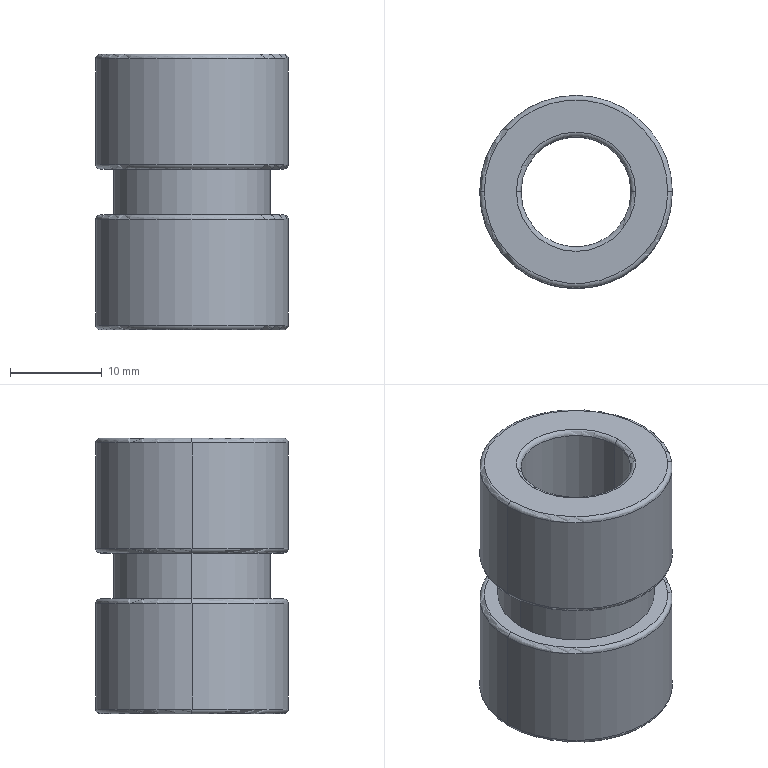Part | SolidWorks | features Extrusion 1, Fillet 1, ICE 1 | 1 solid | 24 faces | box 21 x 21 x 30 mm | volume 6383 mm3 | torus 12 | cylinder 8 | plane 4 | commonest cylinder face diameters 21 x4 12 x2 17 x2
STEP:
#1=CARTESIAN_POINT('',(-10.,0.,2.5));
#2=VERTEX_POINT('',#1);
#3=CARTESIAN_POINT('',(10.,0.,2.5));
#4=VERTEX_POINT('',#3);
#5=CARTESIAN_POINT('',(0.,0.,2.5));
#6=DIRECTION('',(0.,0.,-1.));
#7=DIRECTION('',(1.,0.,0.));
#8=AXIS2_PLACEMENT_3D('',#5,#6,#7);
#9=CIRCLE('',#8,10.);
#10=EDGE_CURVE('',#2,#4,#9,.T.);
#11=ORIENTED_EDGE('',*,*,#10,.F.);
#12=CARTESIAN_POINT('',(-10.5,0.,3.));
#13=VERTEX_POINT('',#12);
#14=CARTESIAN_POINT('',(-10.,0.,3.));
#15=DIRECTION('',(0.,1.,0.));
#16=DIRECTION('',(-1.,0.,0.));
#17=AXIS2_PLACEMENT_3D('',#14,#15,#16);
#18=CIRCLE('',#17,0.5);
#19=EDGE_CURVE('',#2,#13,#18,.T.);
#20=ORIENTED_EDGE('',*,*,#19,.T.);
#21=CARTESIAN_POINT('',(10.5,0.,3.));
#22=VERTEX_POINT('',#21);
#23=CARTESIAN_POINT('',(0.,0.,3.));
#24=DIRECTION('',(0.,0.,1.));
#25=DIRECTION('',(1.,0.,0.));
#26=AXIS2_PLACEMENT_3D('',#23,#24,#25);
#27=CIRCLE('',#26,10.5);
#28=EDGE_CURVE('',#22,#13,#27,.T.);
#29=ORIENTED_EDGE('',*,*,#28,.F.);
#30=CARTESIAN_POINT('',(10.,0.,3.));
#31=DIRECTION('',(0.,-1.,0.));
#32=DIRECTION('',(0.,0.,-1.));
#33=AXIS2_PLACEMENT_3D('',#30,#31,#32);
#34=CIRCLE('',#33,0.5);
#35=EDGE_CURVE('',#4,#22,#34,.T.);
#36=ORIENTED_EDGE('',*,*,#35,.F.);
#37=EDGE_LOOP('',(#11,#20,#29,#36));
#38=FACE_OUTER_BOUND('',#37,.T.);
#39=CARTESIAN_POINT('',(0.,0.,3.));
#40=DIRECTION('',(0.,0.,1.));
#41=DIRECTION('',(1.,0.,0.));
#42=AXIS2_PLACEMENT_3D('',#39,#40,#41);
#43=TOROIDAL_SURFACE('',#42,10.,0.5);
#44=ADVANCED_FACE('',(#38),#43,.T.);
#45=CARTESIAN_POINT('',(-10.5,0.,14.5));
#46=VERTEX_POINT('',#45);
#47=CARTESIAN_POINT('',(10.5,0.,14.5));
#48=VERTEX_POINT('',#47);
#49=CARTESIAN_POINT('',(0.,0.,14.5));
#50=DIRECTION('',(0.,0.,-1.));
#51=DIRECTION('',(1.,0.,0.));
#52=AXIS2_PLACEMENT_3D('',#49,#50,#51);
#53=CIRCLE('',#52,10.5);
#54=EDGE_CURVE('',#46,#48,#53,.T.);
#55=ORIENTED_EDGE('',*,*,#54,.F.);
#56=CARTESIAN_POINT('',(-10.,0.,15.));
#57=VERTEX_POINT('',#56);
#58=CARTESIAN_POINT('',(-10.,0.,14.5));
#59=DIRECTION('',(0.,1.,0.));
#60=DIRECTION('',(-1.,0.,0.));
#61=AXIS2_PLACEMENT_3D('',#58,#59,#60);
#62=CIRCLE('',#61,0.5);
#63=EDGE_CURVE('',#46,#57,#62,.T.);
#64=ORIENTED_EDGE('',*,*,#63,.T.);
#65=CARTESIAN_POINT('',(10.,0.,15.));
#66=VERTEX_POINT('',#65);
#67=CARTESIAN_POINT('',(0.,0.,15.));
#68=DIRECTION('',(0.,0.,1.));
#69=DIRECTION('',(1.,0.,0.));
#70=AXIS2_PLACEMENT_3D('',#67,#68,#69);
#71=CIRCLE('',#70,10.);
#72=EDGE_CURVE('',#66,#57,#71,.T.);
#73=ORIENTED_EDGE('',*,*,#72,.F.);
#74=CARTESIAN_POINT('',(10.,0.,14.5));
#75=DIRECTION('',(0.,-1.,0.));
#76=DIRECTION('',(0.,0.,-1.));
#77=AXIS2_PLACEMENT_3D('',#74,#75,#76);
#78=CIRCLE('',#77,0.5);
#79=EDGE_CURVE('',#48,#66,#78,.T.);
#80=ORIENTED_EDGE('',*,*,#79,.F.);
#81=EDGE_LOOP('',(#55,#64,#73,#80));
#82=FACE_OUTER_BOUND('',#81,.T.);
#83=CARTESIAN_POINT('',(0.,0.,14.5));
#84=DIRECTION('',(0.,0.,1.));
#85=DIRECTION('',(1.,0.,0.));
#86=AXIS2_PLACEMENT_3D('',#83,#84,#85);
#87=TOROIDAL_SURFACE('',#86,10.,0.5);
#88=ADVANCED_FACE('',(#82),#87,.T.);
#89=CARTESIAN_POINT('',(-6.5,0.,15.));
#90=VERTEX_POINT('',#89);
#91=CARTESIAN_POINT('',(6.5,0.,15.));
#92=VERTEX_POINT('',#91);
#93=CARTESIAN_POINT('',(0.,0.,15.));
#94=DIRECTION('',(0.,0.,-1.));
#95=DIRECTION('',(1.,0.,0.));
#96=AXIS2_PLACEMENT_3D('',#93,#94,#95);
#97=CIRCLE('',#96,6.5);
#98=EDGE_CURVE('',#90,#92,#97,.T.);
#99=ORIENTED_EDGE('',*,*,#98,.F.);
#100=CARTESIAN_POINT('',(-6.,0.,14.5));
#101=VERTEX_POINT('',#100);
#102=CARTESIAN_POINT('',(-6.5,0.,14.5));
#103=DIRECTION('',(0.,1.,0.));
#104=DIRECTION('',(-1.,0.,0.));
#105=AXIS2_PLACEMENT_3D('',#102,#103,#104);
#106=CIRCLE('',#105,0.5);
#107=EDGE_CURVE('',#90,#101,#106,.T.);
#108=ORIENTED_EDGE('',*,*,#107,.T.);
#109=CARTESIAN_POINT('',(6.,0.,14.5));
#110=VERTEX_POINT('',#109);
#111=CARTESIAN_POINT('',(0.,0.,14.5));
#112=DIRECTION('',(0.,0.,1.));
#113=DIRECTION('',(1.,0.,0.));
#114=AXIS2_PLACEMENT_3D('',#111,#112,#113);
#115=CIRCLE('',#114,6.);
#116=EDGE_CURVE('',#110,#101,#115,.T.);
#117=ORIENTED_EDGE('',*,*,#116,.F.);
#118=CARTESIAN_POINT('',(6.5,0.,14.5));
#119=DIRECTION('',(0.,-1.,0.));
#120=DIRECTION('',(0.,0.,-1.));
#121=AXIS2_PLACEMENT_3D('',#118,#119,#120);
#122=CIRCLE('',#121,0.5);
#123=EDGE_CURVE('',#92,#110,#122,.T.);
#124=ORIENTED_EDGE('',*,*,#123,.F.);
#125=EDGE_LOOP('',(#99,#108,#117,#124));
#126=FACE_OUTER_BOUND('',#125,.T.);
#127=CARTESIAN_POINT('',(0.,0.,14.5));
#128=DIRECTION('',(0.,0.,1.));
#129=DIRECTION('',(1.,0.,0.));
#130=AXIS2_PLACEMENT_3D('',#127,#128,#129);
#131=TOROIDAL_SURFACE('',#130,6.5,0.5);
#132=ADVANCED_FACE('',(#126),#131,.T.);
#133=CARTESIAN_POINT('',(-6.,0.,-14.5));
#134=VERTEX_POINT('',#133);
#135=CARTESIAN_POINT('',(6.,0.,-14.5));
#136=VERTEX_POINT('',#135);
#137=CARTESIAN_POINT('',(0.,0.,-14.5));
#138=DIRECTION('',(0.,0.,-1.));
#139=DIRECTION('',(1.,0.,0.));
#140=AXIS2_PLACEMENT_3D('',#137,#138,#139);
#141=CIRCLE('',#140,6.);
#142=EDGE_CURVE('',#134,#136,#141,.T.);
#143=ORIENTED_EDGE('',*,*,#142,.F.);
#144=CARTESIAN_POINT('',(-6.5,0.,-15.));
#145=VERTEX_POINT('',#144);
#146=CARTESIAN_POINT('',(-6.5,0.,-14.5));
#147=DIRECTION('',(0.,1.,0.));
#148=DIRECTION('',(-1.,0.,0.));
#149=AXIS2_PLACEMENT_3D('',#146,#147,#148);
#150=CIRCLE('',#149,0.5);
#151=EDGE_CURVE('',#134,#145,#150,.T.);
#152=ORIENTED_EDGE('',*,*,#151,.T.);
#153=CARTESIAN_POINT('',(6.5,0.,-15.));
#154=VERTEX_POINT('',#153);
#155=CARTESIAN_POINT('',(0.,0.,-15.));
#156=DIRECTION('',(0.,0.,1.));
#157=DIRECTION('',(1.,0.,0.));
#158=AXIS2_PLACEMENT_3D('',#155,#156,#157);
#159=CIRCLE('',#158,6.5);
#160=EDGE_CURVE('',#154,#145,#159,.T.);
#161=ORIENTED_EDGE('',*,*,#160,.F.);
#162=CARTESIAN_POINT('',(6.5,0.,-14.5));
#163=DIRECTION('',(0.,-1.,0.));
#164=DIRECTION('',(0.,0.,-1.));
#165=AXIS2_PLACEMENT_3D('',#162,#163,#164);
#166=CIRCLE('',#165,0.5);
#167=EDGE_CURVE('',#136,#154,#166,.T.);
#168=ORIENTED_EDGE('',*,*,#167,.F.);
#169=EDGE_LOOP('',(#143,#152,#161,#168));
#170=FACE_OUTER_BOUND('',#169,.T.);
#171=CARTESIAN_POINT('',(0.,0.,-14.5));
#172=DIRECTION('',(0.,0.,1.));
#173=DIRECTION('',(1.,0.,0.));
#174=AXIS2_PLACEMENT_3D('',#171,#172,#173);
#175=TOROIDAL_SURFACE('',#174,6.5,0.5);
#176=ADVANCED_FACE('',(#170),#175,.T.);
#177=CARTESIAN_POINT('',(-10.,0.,-15.));
#178=VERTEX_POINT('',#177);
#179=CARTESIAN_POINT('',(10.,0.,-15.));
#180=VERTEX_POINT('',#179);
#181=CARTESIAN_POINT('',(0.,0.,-15.));
#182=DIRECTION('',(0.,0.,-1.));
#183=DIRECTION('',(1.,0.,0.));
#184=AXIS2_PLACEMENT_3D('',#181,#182,#183);
#185=CIRCLE('',#184,10.);
#186=EDGE_CURVE('',#178,#180,#185,.T.);
#187=ORIENTED_EDGE('',*,*,#186,.F.);
#188=CARTESIAN_POINT('',(-10.5,0.,-14.5));
#189=VERTEX_POINT('',#188);
#190=CARTESIAN_POINT('',(-10.,0.,-14.5));
#191=DIRECTION('',(0.,1.,0.));
#192=DIRECTION('',(-1.,0.,0.));
#193=AXIS2_PLACEMENT_3D('',#190,#191,#192);
#194=CIRCLE('',#193,0.5);
#195=EDGE_CURVE('',#178,#189,#194,.T.);
#196=ORIENTED_EDGE('',*,*,#195,.T.);
#197=CARTESIAN_POINT('',(10.5,0.,-14.5));
#198=VERTEX_POINT('',#197);
#199=CARTESIAN_POINT('',(0.,0.,-14.5));
#200=DIRECTION('',(0.,0.,1.));
#201=DIRECTION('',(1.,0.,0.));
#202=AXIS2_PLACEMENT_3D('',#199,#200,#201);
#203=CIRCLE('',#202,10.5);
#204=EDGE_CURVE('',#198,#189,#203,.T.);
#205=ORIENTED_EDGE('',*,*,#204,.F.);
#206=CARTESIAN_POINT('',(10.,0.,-14.5));
#207=DIRECTION('',(0.,-1.,0.));
#208=DIRECTION('',(0.,0.,-1.));
#209=AXIS2_PLACEMENT_3D('',#206,#207,#208);
#210=CIRCLE('',#209,0.5);
#211=EDGE_CURVE('',#180,#198,#210,.T.);
#212=ORIENTED_EDGE('',*,*,#211,.F.);
#213=EDGE_LOOP('',(#187,#196,#205,#212));
#214=FACE_OUTER_BOUND('',#213,.T.);
#215=CARTESIAN_POINT('',(0.,0.,-14.5));
#216=DIRECTION('',(0.,0.,1.));
#217=DIRECTION('',(1.,0.,0.));
#218=AXIS2_PLACEMENT_3D('',#215,#216,#217);
#219=TOROIDAL_SURFACE('',#218,10.,0.5);
#220=ADVANCED_FACE('',(#214),#219,.T.);
#221=CARTESIAN_POINT('',(-10.5,0.,-3.));
#222=VERTEX_POINT('',#221);
#223=CARTESIAN_POINT('',(10.5,0.,-3.));
#224=VERTEX_POINT('',#223);
#225=CARTESIAN_POINT('',(0.,0.,-3.));
#226=DIRECTION('',(0.,0.,-1.));
#227=DIRECTION('',(1.,0.,0.));
#228=AXIS2_PLACEMENT_3D('',#225,#226,#227);
#229=CIRCLE('',#228,10.5);
#230=EDGE_CURVE('',#222,#224,#229,.T.);
#231=ORIENTED_EDGE('',*,*,#230,.F.);
#232=CARTESIAN_POINT('',(-10.,0.,-2.5));
#233=VERTEX_POINT('',#232);
#234=CARTESIAN_POINT('',(-10.,0.,-3.));
#235=DIRECTION('',(0.,1.,0.));
#236=DIRECTION('',(-1.,0.,0.));
#237=AXIS2_PLACEMENT_3D('',#234,#235,#236);
#238=CIRCLE('',#237,0.5);
#239=EDGE_CURVE('',#222,#233,#238,.T.);
#240=ORIENTED_EDGE('',*,*,#239,.T.);
#241=CARTESIAN_POINT('',(10.,0.,-2.5));
#242=VERTEX_POINT('',#241);
#243=CARTESIAN_POINT('',(0.,0.,-2.5));
#244=DIRECTION('',(0.,0.,1.));
#245=DIRECTION('',(1.,0.,0.));
#246=AXIS2_PLACEMENT_3D('',#243,#244,#245);
#247=CIRCLE('',#246,10.);
#248=EDGE_CURVE('',#242,#233,#247,.T.);
#249=ORIENTED_EDGE('',*,*,#248,.F.);
#250=CARTESIAN_POINT('',(10.,0.,-3.));
#251=DIRECTION('',(0.,-1.,0.));
#252=DIRECTION('',(0.,0.,-1.));
#253=AXIS2_PLACEMENT_3D('',#250,#251,#252);
#254=CIRCLE('',#253,0.5);
#255=EDGE_CURVE('',#224,#242,#254,.T.);
#256=ORIENTED_EDGE('',*,*,#255,.F.);
#257=EDGE_LOOP('',(#231,#240,#249,#256));
#258=FACE_OUTER_BOUND('',#257,.T.);
#259=CARTESIAN_POINT('',(0.,0.,-3.));
#260=DIRECTION('',(0.,0.,1.));
#261=DIRECTION('',(1.,0.,0.));
#262=AXIS2_PLACEMENT_3D('',#259,#260,#261);
#263=TOROIDAL_SURFACE('',#262,10.,0.5);
#264=ADVANCED_FACE('',(#258),#263,.T.);
#265=CARTESIAN_POINT('',(8.5,0.,-2.5));
#266=VERTEX_POINT('',#265);
#267=CARTESIAN_POINT('',(-8.5,0.,-2.5));
#268=VERTEX_POINT('',#267);
#269=CARTESIAN_POINT('',(0.,0.,-2.5));
#270=DIRECTION('',(0.,0.,1.));
#271=DIRECTION('',(1.,0.,0.));
#272=AXIS2_PLACEMENT_3D('',#269,#270,#271);
#273=CIRCLE('',#272,8.5);
#274=EDGE_CURVE('',#266,#268,#273,.T.);
#275=ORIENTED_EDGE('',*,*,#274,.T.);
#276=CARTESIAN_POINT('',(-8.5,0.,2.5));
#277=VERTEX_POINT('',#276);
#278=CARTESIAN_POINT('',(-8.5,0.,-2.5));
#279=DIRECTION('',(0.,0.,1.));
#280=VECTOR('',#279,1000.);
#281=LINE('',#278,#280);
#282=EDGE_CURVE('',#268,#277,#281,.T.);
#283=ORIENTED_EDGE('',*,*,#282,.T.);
#284=CARTESIAN_POINT('',(8.5,0.,2.5));
#285=VERTEX_POINT('',#284);
#286=CARTESIAN_POINT('',(0.,0.,2.5));
#287=DIRECTION('',(0.,0.,1.));
#288=DIRECTION('',(1.,0.,0.));
#289=AXIS2_PLACEMENT_3D('',#286,#287,#288);
#290=CIRCLE('',#289,8.5);
#291=EDGE_CURVE('',#285,#277,#290,.T.);
#292=ORIENTED_EDGE('',*,*,#291,.F.);
#293=CARTESIAN_POINT('',(8.5,0.,-2.5));
#294=DIRECTION('',(0.,0.,1.));
#295=VECTOR('',#294,1000.);
#296=LINE('',#293,#295);
#297=EDGE_CURVE('',#266,#285,#296,.T.);
#298=ORIENTED_EDGE('',*,*,#297,.F.);
#299=EDGE_LOOP('',(#275,#283,#292,#298));
#300=FACE_OUTER_BOUND('',#299,.T.);
#301=CARTESIAN_POINT('',(0.,0.,-2.5));
#302=DIRECTION('',(0.,0.,1.));
#303=DIRECTION('',(1.,0.,0.));
#304=AXIS2_PLACEMENT_3D('',#301,#302,#303);
#305=CYLINDRICAL_SURFACE('',#304,8.5);
#306=ADVANCED_FACE('',(#300),#305,.T.);
#307=CARTESIAN_POINT('',(0.,0.,14.5));
#308=DIRECTION('',(0.,0.,1.));
#309=DIRECTION('',(1.,0.,0.));
#310=AXIS2_PLACEMENT_3D('',#307,#308,#309);
#311=CIRCLE('',#310,6.);
#312=EDGE_CURVE('',#101,#110,#311,.T.);
#313=ORIENTED_EDGE('',*,*,#312,.T.);
#314=CARTESIAN_POINT('',(6.,0.,15.));
#315=DIRECTION('',(0.,0.,-1.));
#316=VECTOR('',#315,1000.);
#317=LINE('',#314,#316);
#318=EDGE_CURVE('',#110,#136,#317,.T.);
#319=ORIENTED_EDGE('',*,*,#318,.T.);
#320=CARTESIAN_POINT('',(0.,0.,-14.5));
#321=DIRECTION('',(0.,0.,-1.));
#322=DIRECTION('',(1.,0.,0.));
#323=AXIS2_PLACEMENT_3D('',#320,#321,#322);
#324=CIRCLE('',#323,6.);
#325=EDGE_CURVE('',#136,#134,#324,.T.);
#326=ORIENTED_EDGE('',*,*,#325,.T.);
#327=CARTESIAN_POINT('',(-6.,0.,15.));
#328=DIRECTION('',(0.,0.,-1.));
#329=VECTOR('',#328,1000.);
#330=LINE('',#327,#329);
#331=EDGE_CURVE('',#101,#134,#330,.T.);
#332=ORIENTED_EDGE('',*,*,#331,.F.);
#333=EDGE_LOOP('',(#313,#319,#326,#332));
#334=FACE_OUTER_BOUND('',#333,.T.);
#335=CARTESIAN_POINT('',(0.,0.,15.));
#336=DIRECTION('',(0.,0.,-1.));
#337=DIRECTION('',(-1.,0.,0.));
#338=AXIS2_PLACEMENT_3D('',#335,#336,#337);
#339=CYLINDRICAL_SURFACE('',#338,6.);
#340=ADVANCED_FACE('',(#334),#339,.F.);
#341=ORIENTED_EDGE('',*,*,#54,.T.);
#342=CARTESIAN_POINT('',(10.5,0.,15.));
#343=DIRECTION('',(0.,0.,-1.));
#344=VECTOR('',#343,1000.);
#345=LINE('',#342,#344);
#346=EDGE_CURVE('',#48,#22,#345,.T.);
#347=ORIENTED_EDGE('',*,*,#346,.T.);
#348=ORIENTED_EDGE('',*,*,#28,.T.);
#349=CARTESIAN_POINT('',(-10.5,0.,15.));
#350=DIRECTION('',(0.,0.,-1.));
#351=VECTOR('',#350,1000.);
#352=LINE('',#349,#351);
#353=EDGE_CURVE('',#46,#13,#352,.T.);
#354=ORIENTED_EDGE('',*,*,#353,.F.);
#355=EDGE_LOOP('',(#341,#347,#348,#354));
#356=FACE_OUTER_BOUND('',#355,.T.);
#357=CARTESIAN_POINT('',(0.,0.,15.));
#358=DIRECTION('',(0.,0.,-1.));
#359=DIRECTION('',(-1.,0.,0.));
#360=AXIS2_PLACEMENT_3D('',#357,#358,#359);
#361=CYLINDRICAL_SURFACE('',#360,10.5);
#362=ADVANCED_FACE('',(#356),#361,.T.);
#363=ORIENTED_EDGE('',*,*,#230,.T.);
#364=CARTESIAN_POINT('',(10.5,0.,15.));
#365=DIRECTION('',(0.,0.,-1.));
#366=VECTOR('',#365,1000.);
#367=LINE('',#364,#366);
#368=EDGE_CURVE('',#224,#198,#367,.T.);
#369=ORIENTED_EDGE('',*,*,#368,.T.);
#370=ORIENTED_EDGE('',*,*,#204,.T.);
#371=CARTESIAN_POINT('',(-10.5,0.,15.));
#372=DIRECTION('',(0.,0.,-1.));
#373=VECTOR('',#372,1000.);
#374=LINE('',#371,#373);
#375=EDGE_CURVE('',#222,#189,#374,.T.);
#376=ORIENTED_EDGE('',*,*,#375,.F.);
#377=EDGE_LOOP('',(#363,#369,#370,#376));
#378=FACE_OUTER_BOUND('',#377,.T.);
#379=CARTESIAN_POINT('',(0.,0.,15.));
#380=DIRECTION('',(0.,0.,-1.));
#381=DIRECTION('',(-1.,0.,0.));
#382=AXIS2_PLACEMENT_3D('',#379,#380,#381);
#383=CYLINDRICAL_SURFACE('',#382,10.5);
#384=ADVANCED_FACE('',(#378),#383,.T.);
#385=ORIENTED_EDGE('',*,*,#368,.F.);
#386=CARTESIAN_POINT('',(0.,0.,-3.));
#387=DIRECTION('',(0.,0.,-1.));
#388=DIRECTION('',(1.,0.,0.));
#389=AXIS2_PLACEMENT_3D('',#386,#387,#388);
#390=CIRCLE('',#389,10.5);
#391=EDGE_CURVE('',#224,#222,#390,.T.);
#392=ORIENTED_EDGE('',*,*,#391,.T.);
#393=ORIENTED_EDGE('',*,*,#375,.T.);
#394=CARTESIAN_POINT('',(0.,0.,-14.5));
#395=DIRECTION('',(0.,0.,1.));
#396=DIRECTION('',(1.,0.,0.));
#397=AXIS2_PLACEMENT_3D('',#394,#395,#396);
#398=CIRCLE('',#397,10.5);
#399=EDGE_CURVE('',#189,#198,#398,.T.);
#400=ORIENTED_EDGE('',*,*,#399,.T.);
#401=EDGE_LOOP('',(#385,#392,#393,#400));
#402=FACE_OUTER_BOUND('',#401,.T.);
#403=CARTESIAN_POINT('',(0.,0.,15.));
#404=DIRECTION('',(0.,0.,-1.));
#405=DIRECTION('',(-1.,0.,0.));
#406=AXIS2_PLACEMENT_3D('',#403,#404,#405);
#407=CYLINDRICAL_SURFACE('',#406,10.5);
#408=ADVANCED_FACE('',(#402),#407,.T.);
#409=CARTESIAN_POINT('',(0.,0.,15.));
#410=DIRECTION('',(0.,0.,-1.));
#411=DIRECTION('',(1.,0.,0.));
#412=AXIS2_PLACEMENT_3D('',#409,#410,#411);
#413=CIRCLE('',#412,6.5);
#414=EDGE_CURVE('',#92,#90,#413,.T.);
#415=ORIENTED_EDGE('',*,*,#414,.T.);
#416=ORIENTED_EDGE('',*,*,#98,.T.);
#417=EDGE_LOOP('',(#415,#416));
#418=FACE_BOUND('',#417,.T.);
#419=ORIENTED_EDGE('',*,*,#72,.T.);
#420=CARTESIAN_POINT('',(0.,0.,15.));
#421=DIRECTION('',(0.,0.,1.));
#422=DIRECTION('',(1.,0.,0.));
#423=AXIS2_PLACEMENT_3D('',#420,#421,#422);
#424=CIRCLE('',#423,10.);
#425=EDGE_CURVE('',#57,#66,#424,.T.);
#426=ORIENTED_EDGE('',*,*,#425,.T.);
#427=EDGE_LOOP('',(#419,#426));
#428=FACE_OUTER_BOUND('',#427,.T.);
#429=CARTESIAN_POINT('',(0.,0.,15.));
#430=DIRECTION('',(0.,0.,1.));
#431=DIRECTION('',(1.,0.,0.));
#432=AXIS2_PLACEMENT_3D('',#429,#430,#431);
#433=PLANE('',#432);
#434=ADVANCED_FACE('',(#418,#428),#433,.T.);
#435=CARTESIAN_POINT('',(0.,0.,-15.));
#436=DIRECTION('',(0.,0.,-1.));
#437=DIRECTION('',(1.,0.,0.));
#438=AXIS2_PLACEMENT_3D('',#435,#436,#437);
#439=CIRCLE('',#438,10.);
#440=EDGE_CURVE('',#180,#178,#439,.T.);
#441=ORIENTED_EDGE('',*,*,#440,.T.);
#442=ORIENTED_EDGE('',*,*,#186,.T.);
#443=EDGE_LOOP('',(#441,#442));
#444=FACE_OUTER_BOUND('',#443,.T.);
#445=ORIENTED_EDGE('',*,*,#160,.T.);
#446=CARTESIAN_POINT('',(0.,0.,-15.));
#447=DIRECTION('',(0.,0.,1.));
#448=DIRECTION('',(1.,0.,0.));
#449=AXIS2_PLACEMENT_3D('',#446,#447,#448);
#450=CIRCLE('',#449,6.5);
#451=EDGE_CURVE('',#145,#154,#450,.T.);
#452=ORIENTED_EDGE('',*,*,#451,.T.);
#453=EDGE_LOOP('',(#445,#452));
#454=FACE_BOUND('',#453,.T.);
#455=CARTESIAN_POINT('',(0.,0.,-15.));
#456=DIRECTION('',(0.,0.,1.));
#457=DIRECTION('',(1.,0.,0.));
#458=AXIS2_PLACEMENT_3D('',#455,#456,#457);
#459=PLANE('',#458);
#460=ADVANCED_FACE('',(#444,#454),#459,.F.);
#461=ORIENTED_EDGE('',*,*,#346,.F.);
#462=CARTESIAN_POINT('',(0.,0.,14.5));
#463=DIRECTION('',(0.,0.,-1.));
#464=DIRECTION('',(1.,0.,0.));
#465=AXIS2_PLACEMENT_3D('',#462,#463,#464);
#466=CIRCLE('',#465,10.5);
#467=EDGE_CURVE('',#48,#46,#466,.T.);
#468=ORIENTED_EDGE('',*,*,#467,.T.);
#469=ORIENTED_EDGE('',*,*,#353,.T.);
#470=CARTESIAN_POINT('',(0.,0.,3.));
#471=DIRECTION('',(0.,0.,1.));
#472=DIRECTION('',(1.,0.,0.));
#473=AXIS2_PLACEMENT_3D('',#470,#471,#472);
#474=CIRCLE('',#473,10.5);
#475=EDGE_CURVE('',#13,#22,#474,.T.);
#476=ORIENTED_EDGE('',*,*,#475,.T.);
#477=EDGE_LOOP('',(#461,#468,#469,#476));
#478=FACE_OUTER_BOUND('',#477,.T.);
#479=CARTESIAN_POINT('',(0.,0.,15.));
#480=DIRECTION('',(0.,0.,-1.));
#481=DIRECTION('',(-1.,0.,0.));
#482=AXIS2_PLACEMENT_3D('',#479,#480,#481);
#483=CYLINDRICAL_SURFACE('',#482,10.5);
#484=ADVANCED_FACE('',(#478),#483,.T.);
#485=ORIENTED_EDGE('',*,*,#318,.F.);
#486=ORIENTED_EDGE('',*,*,#116,.T.);
#487=ORIENTED_EDGE('',*,*,#331,.T.);
#488=ORIENTED_EDGE('',*,*,#142,.T.);
#489=EDGE_LOOP('',(#485,#486,#487,#488));
#490=FACE_OUTER_BOUND('',#489,.T.);
#491=CARTESIAN_POINT('',(0.,0.,15.));
#492=DIRECTION('',(0.,0.,-1.));
#493=DIRECTION('',(-1.,0.,0.));
#494=AXIS2_PLACEMENT_3D('',#491,#492,#493);
#495=CYLINDRICAL_SURFACE('',#494,6.);
#496=ADVANCED_FACE('',(#490),#495,.F.);
#497=ORIENTED_EDGE('',*,*,#248,.T.);
#498=CARTESIAN_POINT('',(0.,0.,-2.5));
#499=DIRECTION('',(0.,0.,1.));
#500=DIRECTION('',(1.,0.,0.));
#501=AXIS2_PLACEMENT_3D('',#498,#499,#500);
#502=CIRCLE('',#501,10.);
#503=EDGE_CURVE('',#233,#242,#502,.T.);
#504=ORIENTED_EDGE('',*,*,#503,.T.);
#505=EDGE_LOOP('',(#497,#504));
#506=FACE_OUTER_BOUND('',#505,.T.);
#507=ORIENTED_EDGE('',*,*,#274,.F.);
#508=CARTESIAN_POINT('',(0.,0.,-2.5));
#509=DIRECTION('',(0.,0.,1.));
#510=DIRECTION('',(1.,0.,0.));
#511=AXIS2_PLACEMENT_3D('',#508,#509,#510);
#512=CIRCLE('',#511,8.5);
#513=EDGE_CURVE('',#268,#266,#512,.T.);
#514=ORIENTED_EDGE('',*,*,#513,.F.);
#515=EDGE_LOOP('',(#507,#514));
#516=FACE_BOUND('',#515,.T.);
#517=CARTESIAN_POINT('',(0.,0.,-2.5));
#518=DIRECTION('',(0.,0.,1.));
#519=DIRECTION('',(1.,0.,0.));
#520=AXIS2_PLACEMENT_3D('',#517,#518,#519);
#521=PLANE('',#520);
#522=ADVANCED_FACE('',(#506,#516),#521,.T.);
#523=CARTESIAN_POINT('',(0.,0.,2.5));
#524=DIRECTION('',(0.,0.,-1.));
#525=DIRECTION('',(1.,0.,0.));
#526=AXIS2_PLACEMENT_3D('',#523,#524,#525);
#527=CIRCLE('',#526,10.);
#528=EDGE_CURVE('',#4,#2,#527,.T.);
#529=ORIENTED_EDGE('',*,*,#528,.T.);
#530=ORIENTED_EDGE('',*,*,#10,.T.);
#531=EDGE_LOOP('',(#529,#530));
#532=FACE_OUTER_BOUND('',#531,.T.);
#533=ORIENTED_EDGE('',*,*,#291,.T.);
#534=CARTESIAN_POINT('',(0.,0.,2.5));
#535=DIRECTION('',(0.,0.,1.));
#536=DIRECTION('',(1.,0.,0.));
#537=AXIS2_PLACEMENT_3D('',#534,#535,#536);
#538=CIRCLE('',#537,8.5);
#539=EDGE_CURVE('',#277,#285,#538,.T.);
#540=ORIENTED_EDGE('',*,*,#539,.T.);
#541=EDGE_LOOP('',(#533,#540));
#542=FACE_BOUND('',#541,.T.);
#543=CARTESIAN_POINT('',(0.,0.,2.5));
#544=DIRECTION('',(0.,0.,1.));
#545=DIRECTION('',(1.,0.,0.));
#546=AXIS2_PLACEMENT_3D('',#543,#544,#545);
#547=PLANE('',#546);
#548=ADVANCED_FACE('',(#532,#542),#547,.F.);
#549=ORIENTED_EDGE('',*,*,#282,.F.);
#550=ORIENTED_EDGE('',*,*,#513,.T.);
#551=ORIENTED_EDGE('',*,*,#297,.T.);
#552=ORIENTED_EDGE('',*,*,#539,.F.);
#553=EDGE_LOOP('',(#549,#550,#551,#552));
#554=FACE_OUTER_BOUND('',#553,.T.);
#555=CARTESIAN_POINT('',(0.,0.,-2.5));
#556=DIRECTION('',(0.,0.,1.));
#557=DIRECTION('',(1.,0.,0.));
#558=AXIS2_PLACEMENT_3D('',#555,#556,#557);
#559=CYLINDRICAL_SURFACE('',#558,8.5);
#560=ADVANCED_FACE('',(#554),#559,.T.);
#561=ORIENTED_EDGE('',*,*,#239,.F.);
#562=ORIENTED_EDGE('',*,*,#391,.F.);
#563=ORIENTED_EDGE('',*,*,#255,.T.);
#564=ORIENTED_EDGE('',*,*,#503,.F.);
#565=EDGE_LOOP('',(#561,#562,#563,#564));
#566=FACE_OUTER_BOUND('',#565,.T.);
#567=CARTESIAN_POINT('',(0.,0.,-3.));
#568=DIRECTION('',(0.,0.,1.));
#569=DIRECTION('',(1.,0.,0.));
#570=AXIS2_PLACEMENT_3D('',#567,#568,#569);
#571=TOROIDAL_SURFACE('',#570,10.,0.5);
#572=ADVANCED_FACE('',(#566),#571,.T.);
#573=ORIENTED_EDGE('',*,*,#195,.F.);
#574=ORIENTED_EDGE('',*,*,#440,.F.);
#575=ORIENTED_EDGE('',*,*,#211,.T.);
#576=ORIENTED_EDGE('',*,*,#399,.F.);
#577=EDGE_LOOP('',(#573,#574,#575,#576));
#578=FACE_OUTER_BOUND('',#577,.T.);
#579=CARTESIAN_POINT('',(0.,0.,-14.5));
#580=DIRECTION('',(0.,0.,1.));
#581=DIRECTION('',(1.,0.,0.));
#582=AXIS2_PLACEMENT_3D('',#579,#580,#581);
#583=TOROIDAL_SURFACE('',#582,10.,0.5);
#584=ADVANCED_FACE('',(#578),#583,.T.);
#585=ORIENTED_EDGE('',*,*,#151,.F.);
#586=ORIENTED_EDGE('',*,*,#325,.F.);
#587=ORIENTED_EDGE('',*,*,#167,.T.);
#588=ORIENTED_EDGE('',*,*,#451,.F.);
#589=EDGE_LOOP('',(#585,#586,#587,#588));
#590=FACE_OUTER_BOUND('',#589,.T.);
#591=CARTESIAN_POINT('',(0.,0.,-14.5));
#592=DIRECTION('',(0.,0.,1.));
#593=DIRECTION('',(1.,0.,0.));
#594=AXIS2_PLACEMENT_3D('',#591,#592,#593);
#595=TOROIDAL_SURFACE('',#594,6.5,0.5);
#596=ADVANCED_FACE('',(#590),#595,.T.);
#597=ORIENTED_EDGE('',*,*,#107,.F.);
#598=ORIENTED_EDGE('',*,*,#414,.F.);
#599=ORIENTED_EDGE('',*,*,#123,.T.);
#600=ORIENTED_EDGE('',*,*,#312,.F.);
#601=EDGE_LOOP('',(#597,#598,#599,#600));
#602=FACE_OUTER_BOUND('',#601,.T.);
#603=CARTESIAN_POINT('',(0.,0.,14.5));
#604=DIRECTION('',(0.,0.,1.));
#605=DIRECTION('',(1.,0.,0.));
#606=AXIS2_PLACEMENT_3D('',#603,#604,#605);
#607=TOROIDAL_SURFACE('',#606,6.5,0.5);
#608=ADVANCED_FACE('',(#602),#607,.T.);
#609=ORIENTED_EDGE('',*,*,#63,.F.);
#610=ORIENTED_EDGE('',*,*,#467,.F.);
#611=ORIENTED_EDGE('',*,*,#79,.T.);
#612=ORIENTED_EDGE('',*,*,#425,.F.);
#613=EDGE_LOOP('',(#609,#610,#611,#612));
#614=FACE_OUTER_BOUND('',#613,.T.);
#615=CARTESIAN_POINT('',(0.,0.,14.5));
#616=DIRECTION('',(0.,0.,1.));
#617=DIRECTION('',(1.,0.,0.));
#618=AXIS2_PLACEMENT_3D('',#615,#616,#617);
#619=TOROIDAL_SURFACE('',#618,10.,0.5);
#620=ADVANCED_FACE('',(#614),#619,.T.);
#621=ORIENTED_EDGE('',*,*,#19,.F.);
#622=ORIENTED_EDGE('',*,*,#528,.F.);
#623=ORIENTED_EDGE('',*,*,#35,.T.);
#624=ORIENTED_EDGE('',*,*,#475,.F.);
#625=EDGE_LOOP('',(#621,#622,#623,#624));
#626=FACE_OUTER_BOUND('',#625,.T.);
#627=CARTESIAN_POINT('',(0.,0.,3.));
#628=DIRECTION('',(0.,0.,1.));
#629=DIRECTION('',(1.,0.,0.));
#630=AXIS2_PLACEMENT_3D('',#627,#628,#629);
#631=TOROIDAL_SURFACE('',#630,10.,0.5);
#632=ADVANCED_FACE('',(#626),#631,.T.);
#633=CLOSED_SHELL('',(#44,#88,#132,#176,#220,#264,#306,#340,#362,#384,#408,#434,#460,#484,#496,#522,#548,#560,#572,#584,#596,#608,#620,#632));
#634=MANIFOLD_SOLID_BREP('',#633);
#635=CARTESIAN_POINT('',(0.,0.,0.));
#636=DIRECTION('',(0.,0.,1.));
#637=DIRECTION('',(1.,0.,0.));
#638=AXIS2_PLACEMENT_3D('',#635,#636,#637);
#639=(LENGTH_UNIT()NAMED_UNIT(*)SI_UNIT(.MILLI.,.METRE.));
#640=UNCERTAINTY_MEASURE_WITH_UNIT(LENGTH_MEASURE(0.00001),#639,'','');
#641=(NAMED_UNIT(*)PLANE_ANGLE_UNIT()SI_UNIT($,.RADIAN.));
#642=(NAMED_UNIT(*)SI_UNIT($,.STERADIAN.)SOLID_ANGLE_UNIT());
#643=(GEOMETRIC_REPRESENTATION_CONTEXT(3)GLOBAL_UNCERTAINTY_ASSIGNED_CONTEXT((#640))GLOBAL_UNIT_ASSIGNED_CONTEXT((#639,#641,#642))REPRESENTATION_CONTEXT('',''));
#644=ADVANCED_BREP_SHAPE_REPRESENTATION('',(#634,#638),#643);